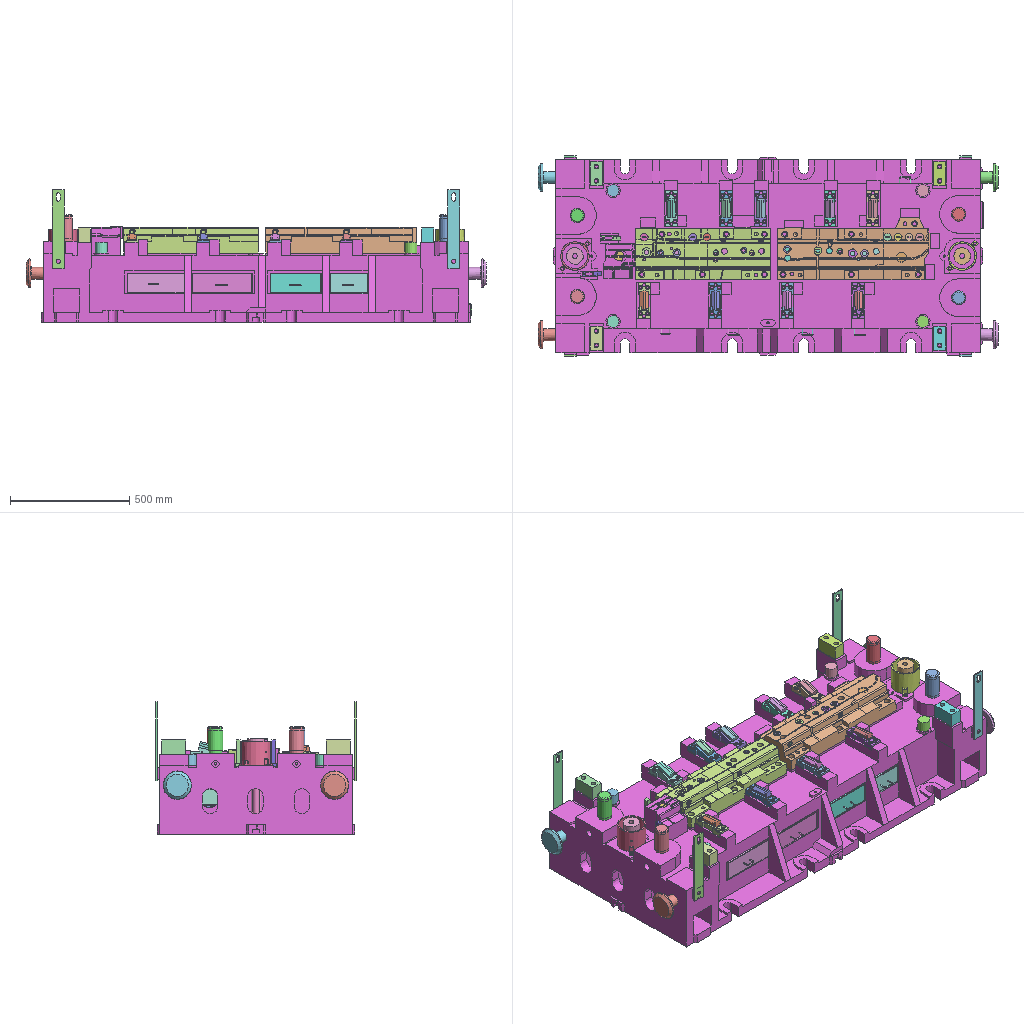Assembly | NX | 123 different items | 123 placed | box 1930 x 840 x 555 mm
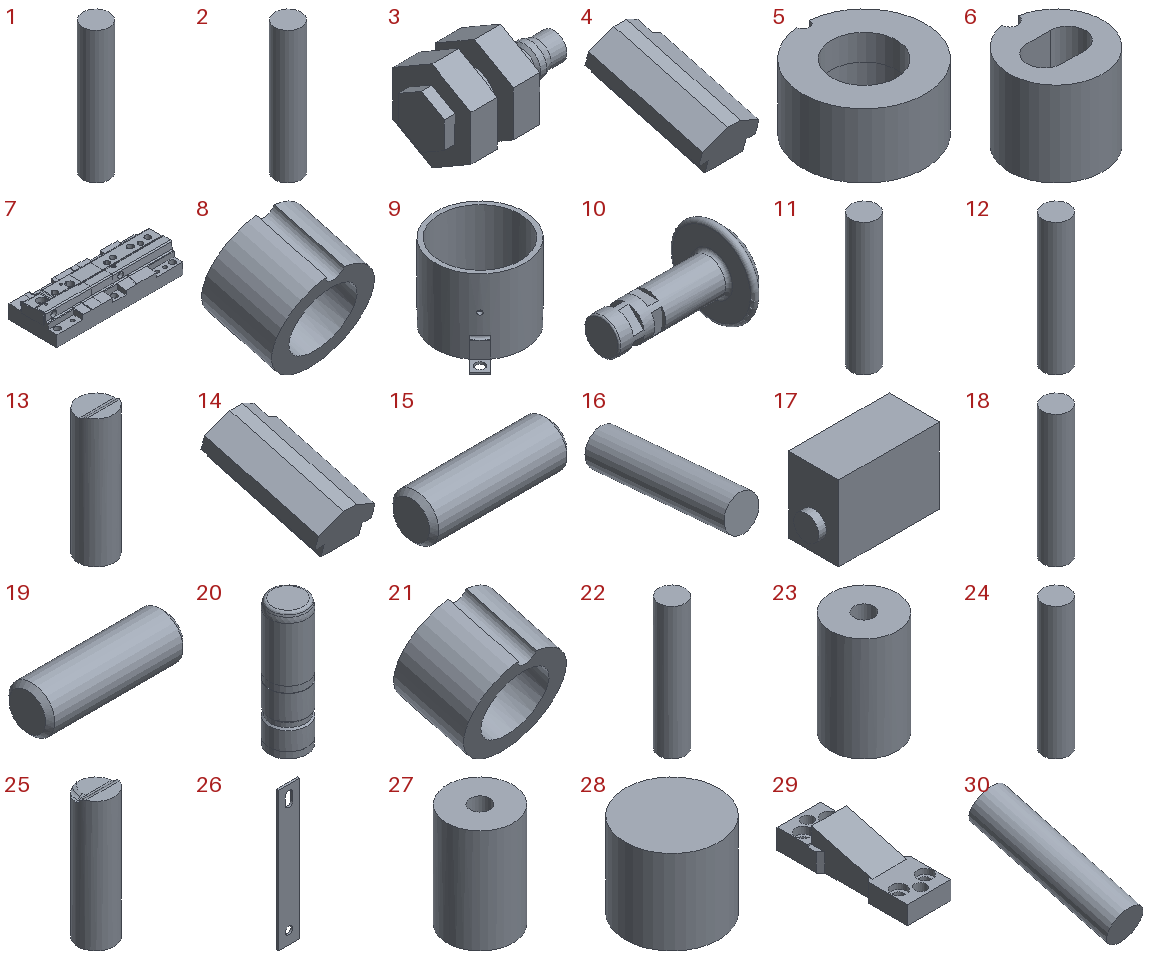Parts list (item | quantity | size | volume | features):
1 | x1 | 4 x 4 x 20 mm | 251.327 mm3 | features solid 2
2 | x1 | 4 x 4 x 20 mm | 251.327 mm3 | features solid 2
3 | x1 | 50 x 29.445 x 34 mm | 18158 mm3 | features solid 2
4 | x1 | 36 x 78.964 x 43.744 mm | 51666 mm3 | features solid 2
5 | x1 | 38 x 37.895 x 20 mm | 15991 mm3 | features solid 2
6 | x1 | 22 x 21.818 x 20 mm | 4687 mm3 | features solid 2
7 | x1 | 570.001 x 220 x 109.482 mm | 7618919 mm3 | features solid 2
8 | x1 | 22 x 21.105 x 25.227 mm | 4030 mm3 | features solid 2
9 | x1 | 134.35 x 134.35 x 100 mm | 216597 mm3 | features solid 2
10 | x1 | 175 x 120 x 120 mm | 487590 mm3 | features solid 2
11 | x1 | 4 x 4 x 20 mm | 251.327 mm3 | features solid 2
12 | x1 | 4 x 4 x 20 mm | 251.327 mm3 | features solid 2
13 | x1 | 40 x 40 x 144.038 mm | 178325 mm3 | features solid 2
14 | x1 | 36 x 78.964 x 43.744 mm | 51666 mm3 | features solid 2
15 | x1 | 30 x 10 x 10 mm | 2327 mm3 | features solid 2
16 | x1 | 4 x 16.288 x 5.379 mm | 201.062 mm3 | features solid 2
17 | x1 | 43 x 20 x 30 mm | 24236 mm3 | features solid 2
18 | x1 | 4 x 4 x 20 mm | 251.327 mm3 | features solid 2
19 | x1 | 30 x 10 x 10 mm | 2327 mm3 | features solid 2
20 | x1 | 60 x 60 x 200 mm | 556815 mm3 | features solid 2
21 | x1 | 22 x 21.105 x 25.227 mm | 4030 mm3 | features solid 2
22 | x1 | 4 x 4 x 20 mm | 251.327 mm3 | features solid 2
23 | x1 | 70 x 70 x 110 mm | 385230 mm3 | features solid 2
24 | x1 | 4 x 4 x 20 mm | 251.327 mm3 | features solid 2
25 | x1 | - | 177258 mm3 | features solid 2
26 | x1 | 50 x 5 x 330 mm | 78425 mm3 | features solid 2
27 | x1 | 70 x 70 x 110 mm | 385230 mm3 | features solid 2
28 | x1 | 50 x 50 x 55 mm | 90902 mm3 | features solid 2
29 | x1 | 50 x 150 x 39.56 mm | 156886 mm3 | features solid 2
30 | x1 | 4 x 16.49 x 8.005 mm | 201.062 mm3 | features solid 2
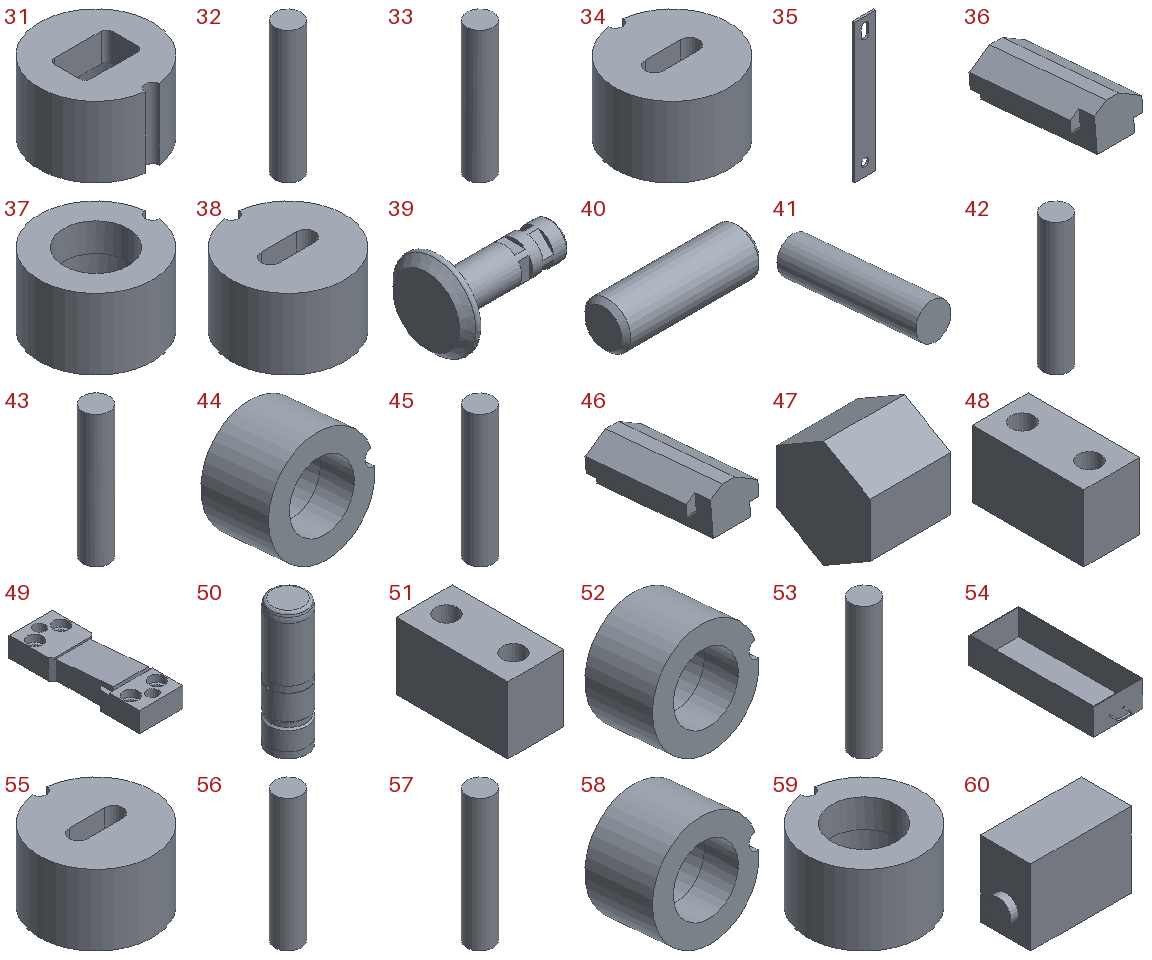31 | x1 | 32 x 31.875 x 20 mm | 10654 mm3 | features solid 2
32 | x1 | 4 x 4 x 20 mm | 251.327 mm3 | features solid 2
33 | x1 | 4 x 4 x 20 mm | 251.327 mm3 | features solid 2
34 | x1 | 32 x 31.875 x 20 mm | 11374 mm3 | features solid 2
35 | x1 | 50 x 5 x 330 mm | 78425 mm3 | features solid 2
36 | x1 | 36 x 76.91 x 31.631 mm | 51666 mm3 | features solid 2
37 | x1 | 31.875 x 32 x 20 mm | 9877 mm3 | features solid 2
38 | x1 | 32 x 31.875 x 20 mm | 11374 mm3 | features solid 2
39 | x1 | 175 x 120 x 120 mm | 487590 mm3 | features solid 2
40 | x1 | 30 x 10 x 10 mm | 2327 mm3 | features solid 2
41 | x1 | 4 x 16.288 x 5.379 mm | 201.062 mm3 | features solid 2
42 | x1 | 4 x 4 x 20 mm | 251.327 mm3 | features solid 2
43 | x1 | 4 x 4 x 20 mm | 251.327 mm3 | features solid 2
44 | x1 | 25 x 18.118 x 26.299 mm | 4570 mm3 | features solid 2
45 | x1 | 4 x 4 x 20 mm | 251.327 mm3 | features solid 2
46 | x1 | 36 x 76.91 x 31.631 mm | 51666 mm3 | features solid 2
47 | x1 | 15 x 17.321 x 20 mm | 3897 mm3 | features solid 2
48 | x1 | 50 x 100 x 60 mm | 268710 mm3 | features solid 2
49 | x1 | 50 x 150 x 26.824 mm | 142519 mm3 | features solid 2
50 | x1 | 60 x 60 x 200 mm | 556815 mm3 | features solid 2
51 | x1 | 50 x 100 x 60 mm | 268710 mm3 | features solid 2
52 | x1 | 25 x 18.118 x 26.299 mm | 4570 mm3 | features solid 2
53 | x1 | 4 x 4 x 20 mm | 251.327 mm3 | features solid 2
54 | x1 | 160 x 429 x 85 mm | 367407 mm3 | features solid 2
55 | x1 | 32 x 31.875 x 20 mm | 11374 mm3 | features solid 2
56 | x1 | 4 x 4 x 20 mm | 251.327 mm3 | features solid 2
57 | x1 | 4 x 4 x 20 mm | 251.327 mm3 | features solid 2
58 | x1 | 25 x 18.118 x 26.299 mm | 4570 mm3 | features solid 2
59 | x1 | 32 x 31.875 x 20 mm | 9877 mm3 | features solid 2
60 | x1 | 43 x 20 x 30 mm | 24236 mm3 | features solid 2
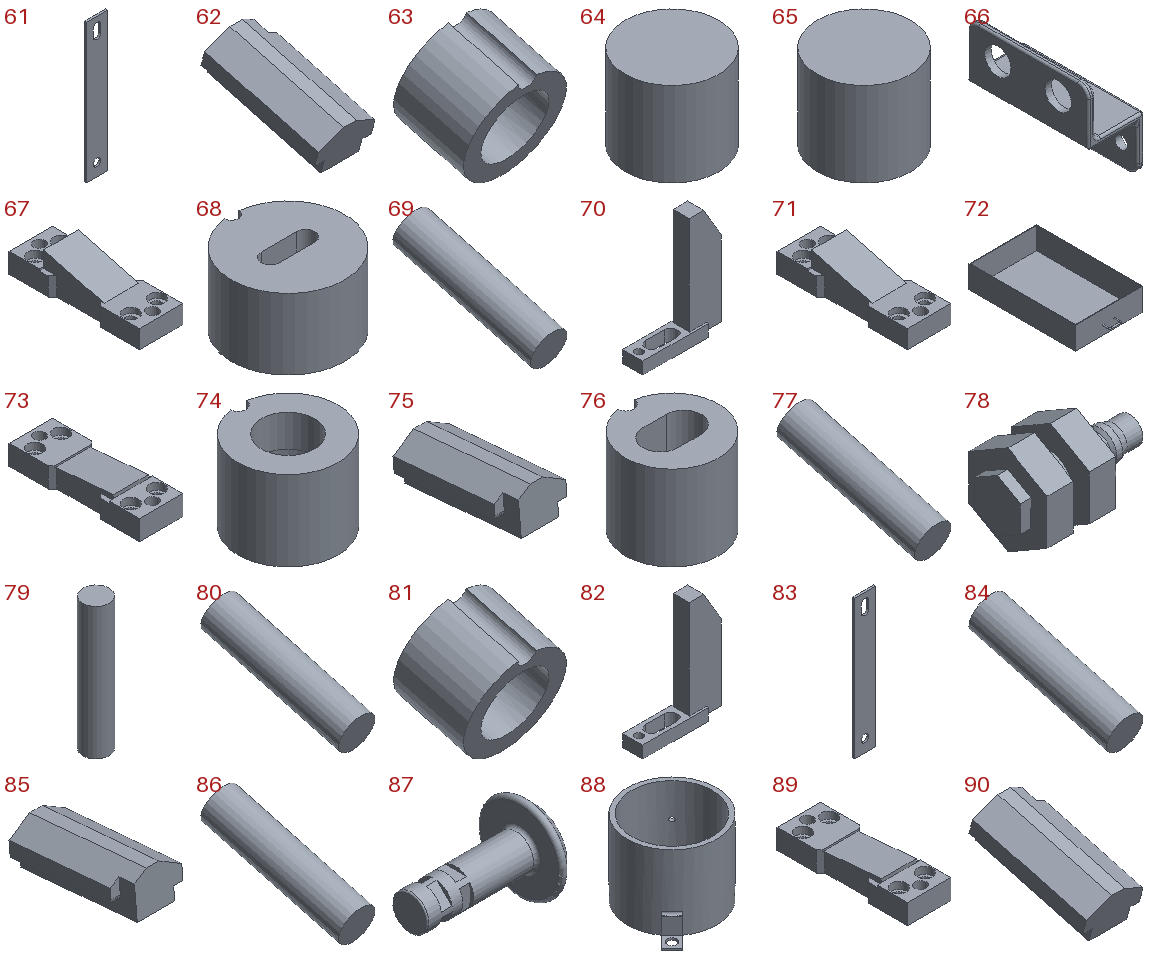61 | x1 | 50 x 5 x 330 mm | 78425 mm3 | features solid 2
62 | x1 | 36 x 78.964 x 43.744 mm | 51666 mm3 | features solid 2
63 | x1 | 22 x 21.102 x 25.216 mm | 4030 mm3 | features solid 2
64 | x1 | 50 x 50 x 55 mm | 90902 mm3 | features solid 2
65 | x1 | 50 x 50 x 55 mm | 90902 mm3 | features solid 2
66 | x1 | 51 x 110 x 93 mm | 84043 mm3 | features solid 2
67 | x1 | 50 x 150 x 39.56 mm | 156886 mm3 | features solid 2
68 | x1 | 32 x 31.875 x 20 mm | 11374 mm3 | features solid 2
69 | x1 | 4 x 16.49 x 8.005 mm | 201.062 mm3 | features solid 2
70 | x1 | 80 x 20 x 110 mm | 58169 mm3 | features solid 2
71 | x1 | 50 x 150 x 39.56 mm | 156886 mm3 | features solid 2
72 | x1 | 255 x 429 x 85 mm | 497676 mm3 | features solid 2
73 | x1 | 50 x 150 x 26.824 mm | 142519 mm3 | features solid 2
74 | x1 | 25 x 24.84 x 20 mm | 5998 mm3 | features solid 2
75 | x1 | 36 x 76.91 x 31.631 mm | 51666 mm3 | features solid 2
76 | x1 | 22 x 21.818 x 20 mm | 4687 mm3 | features solid 2
77 | x1 | 4 x 16.49 x 8.005 mm | 201.062 mm3 | features solid 2
78 | x1 | 50 x 29.445 x 34 mm | 18158 mm3 | features solid 2
79 | x1 | 4 x 4 x 20 mm | 251.327 mm3 | features solid 2
80 | x1 | 4 x 16.49 x 8.005 mm | 201.062 mm3 | features solid 2
81 | x1 | 22 x 21.105 x 25.227 mm | 4030 mm3 | features solid 2
82 | x1 | 80 x 20 x 110 mm | 58169 mm3 | features solid 2
83 | x1 | 50 x 5 x 330 mm | 78425 mm3 | features solid 2
84 | x1 | 4 x 16.49 x 8.005 mm | 201.062 mm3 | features solid 2
85 | x1 | 36 x 76.91 x 31.631 mm | 51666 mm3 | features solid 2
86 | x1 | 4 x 16.49 x 8.005 mm | 201.062 mm3 | features solid 2
87 | x1 | 175 x 120 x 120 mm | 487590 mm3 | features solid 2
88 | x1 | 134.35 x 134.35 x 100 mm | 216597 mm3 | features solid 2
89 | x1 | 50 x 150 x 26.824 mm | 142519 mm3 | features solid 2
90 | x1 | 36 x 78.964 x 43.744 mm | 51666 mm3 | features solid 2
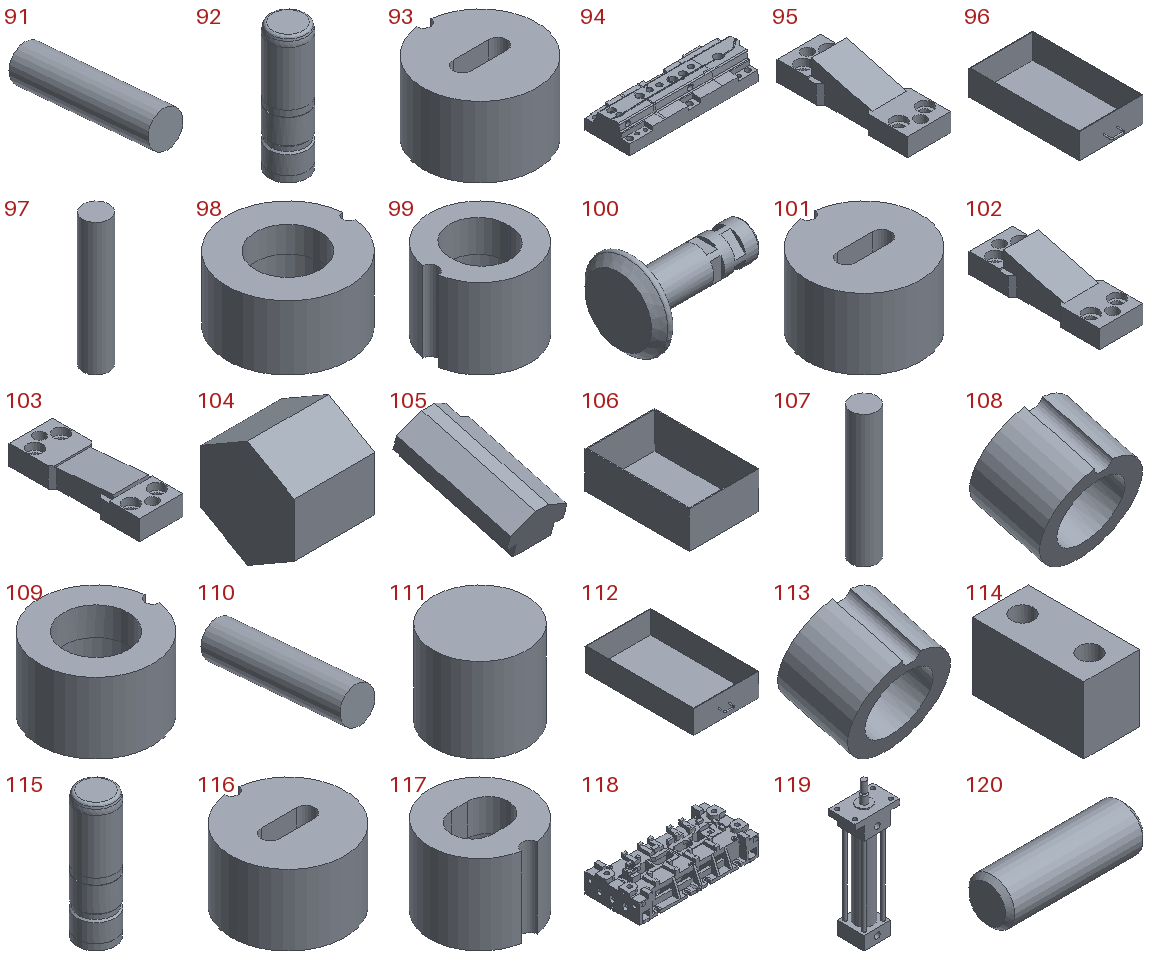91 | x1 | 4 x 16.288 x 5.379 mm | 201.062 mm3 | features solid 2
92 | x1 | 60 x 60 x 200 mm | 556815 mm3 | features solid 2
93 | x1 | 32 x 31.875 x 20 mm | 11374 mm3 | features solid 2
94 | x1 | 640 x 260 x 108.199 mm | 8623447 mm3 | features solid 2
95 | x1 | 50 x 150 x 39.56 mm | 156886 mm3 | features solid 2
96 | x1 | 215 x 399 x 85 mm | 439303 mm3 | features solid 2
97 | x1 | 4 x 4 x 20 mm | 251.327 mm3 | features solid 2
98 | x1 | 37.895 x 38 x 20 mm | 15991 mm3 | features solid 2
99 | x1 | 24.84 x 25 x 20 mm | 5715 mm3 | features solid 2
100 | x1 | 175 x 120 x 120 mm | 487590 mm3 | features solid 2
101 | x1 | 32 x 31.875 x 20 mm | 11374 mm3 | features solid 2
102 | x1 | 50 x 150 x 39.56 mm | 156886 mm3 | features solid 2
103 | x1 | 50 x 150 x 26.824 mm | 142519 mm3 | features solid 2
104 | x1 | 15 x 17.321 x 20 mm | 3897 mm3 | features solid 2
105 | x1 | 36 x 78.964 x 43.744 mm | 51666 mm3 | features solid 2
106 | x1 | 160 x 269 x 85 mm | 244007 mm3 | features solid 2
107 | x1 | 4 x 4 x 20 mm | 251.327 mm3 | features solid 2
108 | x1 | 22 x 21.102 x 25.216 mm | 4030 mm3 | features solid 2
109 | x1 | 31.875 x 32 x 20 mm | 9877 mm3 | features solid 2
110 | x1 | 4 x 16.288 x 5.379 mm | 201.062 mm3 | features solid 2
111 | x1 | 50 x 50 x 55 mm | 90902 mm3 | features solid 2
112 | x1 | 240 x 425 x 85 mm | 476906 mm3 | features solid 2
113 | x1 | 22 x 21.102 x 25.216 mm | 4030 mm3 | features solid 2
114 | x1 | 50 x 100 x 60 mm | 268710 mm3 | features solid 2
115 | x1 | 60 x 60 x 200 mm | 556815 mm3 | features solid 2
116 | x1 | 32 x 31.875 x 20 mm | 11374 mm3 | features solid 2
117 | x1 | 25 x 24.84 x 20 mm | 6116 mm3 | features solid 2
118 | x1 | 1800 x 830 x 402.213 mm | 167101651 mm3 | features solid 2
119 | x1 | 80 x 48 x 245 mm | 201071 mm3 | features solid 2
120 | x1 | 30 x 10 x 10 mm | 2327 mm3 | features solid 2
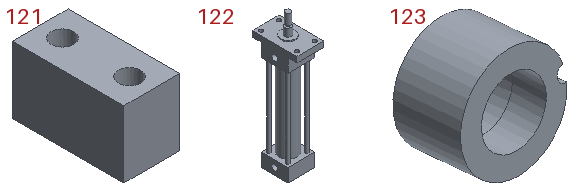121 | x1 | 50 x 100 x 60 mm | 268710 mm3 | features solid 2
122 | x1 | 48 x 80 x 245 mm | 201071 mm3 | features solid 2
123 | x1 | 25 x 18.118 x 26.299 mm | 4570 mm3 | features solid 2